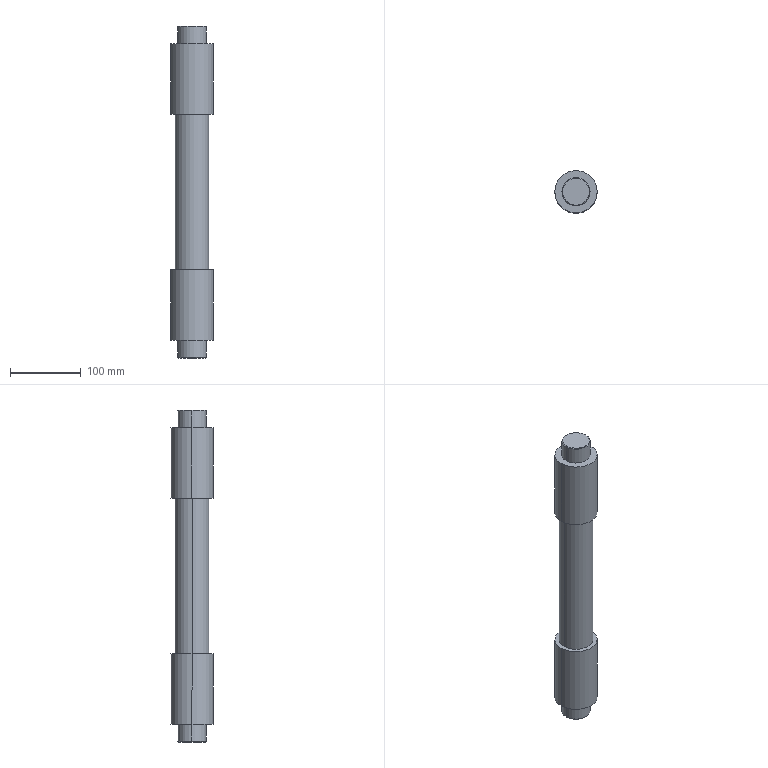Part | SolidWorks | features ICE 2, RevCut 2, Extrusion 1 | 1 solid | 20 faces | box 60 x 60 x 470 mm | volume 1026298 mm3 | cylinder 10 | plane 6 | cone 4 | commonest cylinder face diameters 40 x4 60 x4 48 x2
STEP:
#1=CARTESIAN_POINT('',(19.,0.,0.));
#2=VERTEX_POINT('',#1);
#3=CARTESIAN_POINT('',(-19.,0.,0.));
#4=VERTEX_POINT('',#3);
#5=CARTESIAN_POINT('',(0.,0.,0.));
#6=DIRECTION('',(0.,0.,1.));
#7=DIRECTION('',(1.,0.,0.));
#8=AXIS2_PLACEMENT_3D('',#5,#6,#7);
#9=CIRCLE('',#8,19.);
#10=EDGE_CURVE('',#2,#4,#9,.T.);
#11=ORIENTED_EDGE('',*,*,#10,.T.);
#12=CARTESIAN_POINT('',(-20.,0.,1.));
#13=VERTEX_POINT('',#12);
#14=CARTESIAN_POINT('',(-20.,0.,1.));
#15=DIRECTION('',(-0.7071,0.,0.7071));
#16=VECTOR('',#15,1000.);
#17=LINE('',#14,#16);
#18=EDGE_CURVE('',#4,#13,#17,.T.);
#19=ORIENTED_EDGE('',*,*,#18,.T.);
#20=CARTESIAN_POINT('',(20.,0.,1.));
#21=VERTEX_POINT('',#20);
#22=CARTESIAN_POINT('',(0.,0.,1.));
#23=DIRECTION('',(0.,0.,1.));
#24=DIRECTION('',(1.,0.,0.));
#25=AXIS2_PLACEMENT_3D('',#22,#23,#24);
#26=CIRCLE('',#25,20.);
#27=EDGE_CURVE('',#21,#13,#26,.T.);
#28=ORIENTED_EDGE('',*,*,#27,.F.);
#29=CARTESIAN_POINT('',(20.,0.,1.));
#30=DIRECTION('',(0.7071,0.,0.7071));
#31=VECTOR('',#30,1000.);
#32=LINE('',#29,#31);
#33=EDGE_CURVE('',#2,#21,#32,.T.);
#34=ORIENTED_EDGE('',*,*,#33,.F.);
#35=EDGE_LOOP('',(#11,#19,#28,#34));
#36=FACE_OUTER_BOUND('',#35,.T.);
#37=CARTESIAN_POINT('',(0.,0.,1.));
#38=DIRECTION('',(0.,0.,1.));
#39=DIRECTION('',(1.,0.,0.));
#40=AXIS2_PLACEMENT_3D('',#37,#38,#39);
#41=CONICAL_SURFACE('',#40,20.,0.7854);
#42=ADVANCED_FACE('',(#36),#41,.T.);
#43=CARTESIAN_POINT('',(19.,0.,470.));
#44=VERTEX_POINT('',#43);
#45=CARTESIAN_POINT('',(-19.,0.,470.));
#46=VERTEX_POINT('',#45);
#47=CARTESIAN_POINT('',(0.,0.,470.));
#48=DIRECTION('',(0.,0.,1.));
#49=DIRECTION('',(1.,0.,0.));
#50=AXIS2_PLACEMENT_3D('',#47,#48,#49);
#51=CIRCLE('',#50,19.);
#52=EDGE_CURVE('',#44,#46,#51,.T.);
#53=ORIENTED_EDGE('',*,*,#52,.F.);
#54=CARTESIAN_POINT('',(20.,0.,469.));
#55=VERTEX_POINT('',#54);
#56=CARTESIAN_POINT('',(20.,0.,469.));
#57=DIRECTION('',(0.7071,0.,-0.7071));
#58=VECTOR('',#57,1000.);
#59=LINE('',#56,#58);
#60=EDGE_CURVE('',#44,#55,#59,.T.);
#61=ORIENTED_EDGE('',*,*,#60,.T.);
#62=CARTESIAN_POINT('',(-20.,0.,469.));
#63=VERTEX_POINT('',#62);
#64=CARTESIAN_POINT('',(0.,0.,469.));
#65=DIRECTION('',(0.,0.,1.));
#66=DIRECTION('',(1.,0.,0.));
#67=AXIS2_PLACEMENT_3D('',#64,#65,#66);
#68=CIRCLE('',#67,20.);
#69=EDGE_CURVE('',#55,#63,#68,.T.);
#70=ORIENTED_EDGE('',*,*,#69,.T.);
#71=CARTESIAN_POINT('',(-20.,0.,469.));
#72=DIRECTION('',(-0.7071,0.,-0.7071));
#73=VECTOR('',#72,1000.);
#74=LINE('',#71,#73);
#75=EDGE_CURVE('',#46,#63,#74,.T.);
#76=ORIENTED_EDGE('',*,*,#75,.F.);
#77=EDGE_LOOP('',(#53,#61,#70,#76));
#78=FACE_OUTER_BOUND('',#77,.T.);
#79=CARTESIAN_POINT('',(0.,0.,469.));
#80=DIRECTION('',(0.,0.,-1.));
#81=DIRECTION('',(-1.,0.,0.));
#82=AXIS2_PLACEMENT_3D('',#79,#80,#81);
#83=CONICAL_SURFACE('',#82,20.,0.7854);
#84=ADVANCED_FACE('',(#78),#83,.T.);
#85=CARTESIAN_POINT('',(30.,0.,125.));
#86=VERTEX_POINT('',#85);
#87=CARTESIAN_POINT('',(-30.,0.,125.));
#88=VERTEX_POINT('',#87);
#89=CARTESIAN_POINT('',(0.,0.,125.));
#90=DIRECTION('',(0.,0.,1.));
#91=DIRECTION('',(1.,0.,0.));
#92=AXIS2_PLACEMENT_3D('',#89,#90,#91);
#93=CIRCLE('',#92,30.);
#94=EDGE_CURVE('',#86,#88,#93,.T.);
#95=ORIENTED_EDGE('',*,*,#94,.F.);
#96=CARTESIAN_POINT('',(30.,0.,25.));
#97=VERTEX_POINT('',#96);
#98=CARTESIAN_POINT('',(30.,0.,470.));
#99=DIRECTION('',(0.,0.,-1.));
#100=VECTOR('',#99,1000.);
#101=LINE('',#98,#100);
#102=EDGE_CURVE('',#86,#97,#101,.T.);
#103=ORIENTED_EDGE('',*,*,#102,.T.);
#104=CARTESIAN_POINT('',(-30.,0.,25.));
#105=VERTEX_POINT('',#104);
#106=CARTESIAN_POINT('',(0.,0.,25.));
#107=DIRECTION('',(0.,0.,-1.));
#108=DIRECTION('',(-1.,0.,0.));
#109=AXIS2_PLACEMENT_3D('',#106,#107,#108);
#110=CIRCLE('',#109,30.);
#111=EDGE_CURVE('',#105,#97,#110,.T.);
#112=ORIENTED_EDGE('',*,*,#111,.F.);
#113=CARTESIAN_POINT('',(-30.,0.,470.));
#114=DIRECTION('',(0.,0.,-1.));
#115=VECTOR('',#114,1000.);
#116=LINE('',#113,#115);
#117=EDGE_CURVE('',#88,#105,#116,.T.);
#118=ORIENTED_EDGE('',*,*,#117,.F.);
#119=EDGE_LOOP('',(#95,#103,#112,#118));
#120=FACE_OUTER_BOUND('',#119,.T.);
#121=CARTESIAN_POINT('',(0.,0.,470.));
#122=DIRECTION('',(0.,0.,-1.));
#123=DIRECTION('',(-1.,0.,0.));
#124=AXIS2_PLACEMENT_3D('',#121,#122,#123);
#125=CYLINDRICAL_SURFACE('',#124,30.);
#126=ADVANCED_FACE('',(#120),#125,.T.);
#127=CARTESIAN_POINT('',(24.,0.,125.));
#128=VERTEX_POINT('',#127);
#129=CARTESIAN_POINT('',(-24.,0.,125.));
#130=VERTEX_POINT('',#129);
#131=CARTESIAN_POINT('',(0.,0.,125.));
#132=DIRECTION('',(0.,0.,1.));
#133=DIRECTION('',(1.,0.,0.));
#134=AXIS2_PLACEMENT_3D('',#131,#132,#133);
#135=CIRCLE('',#134,24.);
#136=EDGE_CURVE('',#128,#130,#135,.T.);
#137=ORIENTED_EDGE('',*,*,#136,.T.);
#138=CARTESIAN_POINT('',(-24.,0.,345.));
#139=VERTEX_POINT('',#138);
#140=CARTESIAN_POINT('',(-24.,0.,345.));
#141=DIRECTION('',(0.,0.,1.));
#142=VECTOR('',#141,1000.);
#143=LINE('',#140,#142);
#144=EDGE_CURVE('',#130,#139,#143,.T.);
#145=ORIENTED_EDGE('',*,*,#144,.T.);
#146=CARTESIAN_POINT('',(24.,0.,345.));
#147=VERTEX_POINT('',#146);
#148=CARTESIAN_POINT('',(0.,0.,345.));
#149=DIRECTION('',(0.,0.,1.));
#150=DIRECTION('',(1.,0.,0.));
#151=AXIS2_PLACEMENT_3D('',#148,#149,#150);
#152=CIRCLE('',#151,24.);
#153=EDGE_CURVE('',#147,#139,#152,.T.);
#154=ORIENTED_EDGE('',*,*,#153,.F.);
#155=CARTESIAN_POINT('',(24.,0.,345.));
#156=DIRECTION('',(0.,0.,1.));
#157=VECTOR('',#156,1000.);
#158=LINE('',#155,#157);
#159=EDGE_CURVE('',#128,#147,#158,.T.);
#160=ORIENTED_EDGE('',*,*,#159,.F.);
#161=EDGE_LOOP('',(#137,#145,#154,#160));
#162=FACE_OUTER_BOUND('',#161,.T.);
#163=CARTESIAN_POINT('',(0.,0.,345.));
#164=DIRECTION('',(0.,0.,1.));
#165=DIRECTION('',(1.,0.,0.));
#166=AXIS2_PLACEMENT_3D('',#163,#164,#165);
#167=CYLINDRICAL_SURFACE('',#166,24.);
#168=ADVANCED_FACE('',(#162),#167,.T.);
#169=CARTESIAN_POINT('',(20.,0.,445.));
#170=VERTEX_POINT('',#169);
#171=CARTESIAN_POINT('',(-20.,0.,445.));
#172=VERTEX_POINT('',#171);
#173=CARTESIAN_POINT('',(0.,0.,445.));
#174=DIRECTION('',(0.,0.,1.));
#175=DIRECTION('',(1.,0.,0.));
#176=AXIS2_PLACEMENT_3D('',#173,#174,#175);
#177=CIRCLE('',#176,20.);
#178=EDGE_CURVE('',#170,#172,#177,.T.);
#179=ORIENTED_EDGE('',*,*,#178,.T.);
#180=CARTESIAN_POINT('',(-20.,0.,445.));
#181=DIRECTION('',(0.,0.,1.));
#182=VECTOR('',#181,1000.);
#183=LINE('',#180,#182);
#184=EDGE_CURVE('',#172,#63,#183,.T.);
#185=ORIENTED_EDGE('',*,*,#184,.T.);
#186=ORIENTED_EDGE('',*,*,#69,.F.);
#187=CARTESIAN_POINT('',(20.,0.,445.));
#188=DIRECTION('',(0.,0.,1.));
#189=VECTOR('',#188,1000.);
#190=LINE('',#187,#189);
#191=EDGE_CURVE('',#170,#55,#190,.T.);
#192=ORIENTED_EDGE('',*,*,#191,.F.);
#193=EDGE_LOOP('',(#179,#185,#186,#192));
#194=FACE_OUTER_BOUND('',#193,.T.);
#195=CARTESIAN_POINT('',(0.,0.,445.));
#196=DIRECTION('',(0.,0.,1.));
#197=DIRECTION('',(1.,0.,0.));
#198=AXIS2_PLACEMENT_3D('',#195,#196,#197);
#199=CYLINDRICAL_SURFACE('',#198,20.);
#200=ADVANCED_FACE('',(#194),#199,.T.);
#201=CARTESIAN_POINT('',(30.,0.,445.));
#202=VERTEX_POINT('',#201);
#203=CARTESIAN_POINT('',(-30.,0.,445.));
#204=VERTEX_POINT('',#203);
#205=CARTESIAN_POINT('',(0.,0.,445.));
#206=DIRECTION('',(0.,0.,1.));
#207=DIRECTION('',(1.,0.,0.));
#208=AXIS2_PLACEMENT_3D('',#205,#206,#207);
#209=CIRCLE('',#208,30.);
#210=EDGE_CURVE('',#202,#204,#209,.T.);
#211=ORIENTED_EDGE('',*,*,#210,.F.);
#212=CARTESIAN_POINT('',(30.,0.,345.));
#213=VERTEX_POINT('',#212);
#214=CARTESIAN_POINT('',(30.,0.,470.));
#215=DIRECTION('',(0.,0.,-1.));
#216=VECTOR('',#215,1000.);
#217=LINE('',#214,#216);
#218=EDGE_CURVE('',#202,#213,#217,.T.);
#219=ORIENTED_EDGE('',*,*,#218,.T.);
#220=CARTESIAN_POINT('',(-30.,0.,345.));
#221=VERTEX_POINT('',#220);
#222=CARTESIAN_POINT('',(0.,0.,345.));
#223=DIRECTION('',(0.,0.,1.));
#224=DIRECTION('',(1.,0.,0.));
#225=AXIS2_PLACEMENT_3D('',#222,#223,#224);
#226=CIRCLE('',#225,30.);
#227=EDGE_CURVE('',#213,#221,#226,.T.);
#228=ORIENTED_EDGE('',*,*,#227,.T.);
#229=CARTESIAN_POINT('',(-30.,0.,470.));
#230=DIRECTION('',(0.,0.,-1.));
#231=VECTOR('',#230,1000.);
#232=LINE('',#229,#231);
#233=EDGE_CURVE('',#204,#221,#232,.T.);
#234=ORIENTED_EDGE('',*,*,#233,.F.);
#235=EDGE_LOOP('',(#211,#219,#228,#234));
#236=FACE_OUTER_BOUND('',#235,.T.);
#237=CARTESIAN_POINT('',(0.,0.,470.));
#238=DIRECTION('',(0.,0.,-1.));
#239=DIRECTION('',(-1.,0.,0.));
#240=AXIS2_PLACEMENT_3D('',#237,#238,#239);
#241=CYLINDRICAL_SURFACE('',#240,30.);
#242=ADVANCED_FACE('',(#236),#241,.T.);
#243=CARTESIAN_POINT('',(-20.,0.,25.));
#244=VERTEX_POINT('',#243);
#245=CARTESIAN_POINT('',(20.,0.,25.));
#246=VERTEX_POINT('',#245);
#247=CARTESIAN_POINT('',(0.,0.,25.));
#248=DIRECTION('',(0.,0.,-1.));
#249=DIRECTION('',(-1.,0.,0.));
#250=AXIS2_PLACEMENT_3D('',#247,#248,#249);
#251=CIRCLE('',#250,20.);
#252=EDGE_CURVE('',#244,#246,#251,.T.);
#253=ORIENTED_EDGE('',*,*,#252,.T.);
#254=CARTESIAN_POINT('',(20.,0.,25.));
#255=DIRECTION('',(0.,0.,-1.));
#256=VECTOR('',#255,1000.);
#257=LINE('',#254,#256);
#258=EDGE_CURVE('',#246,#21,#257,.T.);
#259=ORIENTED_EDGE('',*,*,#258,.T.);
#260=ORIENTED_EDGE('',*,*,#27,.T.);
#261=CARTESIAN_POINT('',(-20.,0.,25.));
#262=DIRECTION('',(0.,0.,-1.));
#263=VECTOR('',#262,1000.);
#264=LINE('',#261,#263);
#265=EDGE_CURVE('',#244,#13,#264,.T.);
#266=ORIENTED_EDGE('',*,*,#265,.F.);
#267=EDGE_LOOP('',(#253,#259,#260,#266));
#268=FACE_OUTER_BOUND('',#267,.T.);
#269=CARTESIAN_POINT('',(0.,0.,25.));
#270=DIRECTION('',(0.,0.,-1.));
#271=DIRECTION('',(-1.,0.,0.));
#272=AXIS2_PLACEMENT_3D('',#269,#270,#271);
#273=CYLINDRICAL_SURFACE('',#272,20.);
#274=ADVANCED_FACE('',(#268),#273,.T.);
#275=ORIENTED_EDGE('',*,*,#258,.F.);
#276=CARTESIAN_POINT('',(0.,0.,25.));
#277=DIRECTION('',(0.,0.,-1.));
#278=DIRECTION('',(-1.,0.,0.));
#279=AXIS2_PLACEMENT_3D('',#276,#277,#278);
#280=CIRCLE('',#279,20.);
#281=EDGE_CURVE('',#246,#244,#280,.T.);
#282=ORIENTED_EDGE('',*,*,#281,.T.);
#283=ORIENTED_EDGE('',*,*,#265,.T.);
#284=CARTESIAN_POINT('',(0.,0.,1.));
#285=DIRECTION('',(0.,0.,1.));
#286=DIRECTION('',(1.,0.,0.));
#287=AXIS2_PLACEMENT_3D('',#284,#285,#286);
#288=CIRCLE('',#287,20.);
#289=EDGE_CURVE('',#13,#21,#288,.T.);
#290=ORIENTED_EDGE('',*,*,#289,.T.);
#291=EDGE_LOOP('',(#275,#282,#283,#290));
#292=FACE_OUTER_BOUND('',#291,.T.);
#293=CARTESIAN_POINT('',(0.,0.,25.));
#294=DIRECTION('',(0.,0.,-1.));
#295=DIRECTION('',(-1.,0.,0.));
#296=AXIS2_PLACEMENT_3D('',#293,#294,#295);
#297=CYLINDRICAL_SURFACE('',#296,20.);
#298=ADVANCED_FACE('',(#292),#297,.T.);
#299=ORIENTED_EDGE('',*,*,#218,.F.);
#300=CARTESIAN_POINT('',(0.,0.,445.));
#301=DIRECTION('',(0.,0.,1.));
#302=DIRECTION('',(1.,0.,0.));
#303=AXIS2_PLACEMENT_3D('',#300,#301,#302);
#304=CIRCLE('',#303,30.);
#305=EDGE_CURVE('',#204,#202,#304,.T.);
#306=ORIENTED_EDGE('',*,*,#305,.F.);
#307=ORIENTED_EDGE('',*,*,#233,.T.);
#308=CARTESIAN_POINT('',(0.,0.,345.));
#309=DIRECTION('',(0.,0.,1.));
#310=DIRECTION('',(1.,0.,0.));
#311=AXIS2_PLACEMENT_3D('',#308,#309,#310);
#312=CIRCLE('',#311,30.);
#313=EDGE_CURVE('',#221,#213,#312,.T.);
#314=ORIENTED_EDGE('',*,*,#313,.T.);
#315=EDGE_LOOP('',(#299,#306,#307,#314));
#316=FACE_OUTER_BOUND('',#315,.T.);
#317=CARTESIAN_POINT('',(0.,0.,470.));
#318=DIRECTION('',(0.,0.,-1.));
#319=DIRECTION('',(-1.,0.,0.));
#320=AXIS2_PLACEMENT_3D('',#317,#318,#319);
#321=CYLINDRICAL_SURFACE('',#320,30.);
#322=ADVANCED_FACE('',(#316),#321,.T.);
#323=ORIENTED_EDGE('',*,*,#178,.F.);
#324=CARTESIAN_POINT('',(0.,0.,445.));
#325=DIRECTION('',(0.,0.,1.));
#326=DIRECTION('',(1.,0.,0.));
#327=AXIS2_PLACEMENT_3D('',#324,#325,#326);
#328=CIRCLE('',#327,20.);
#329=EDGE_CURVE('',#172,#170,#328,.T.);
#330=ORIENTED_EDGE('',*,*,#329,.F.);
#331=EDGE_LOOP('',(#323,#330));
#332=FACE_BOUND('',#331,.T.);
#333=ORIENTED_EDGE('',*,*,#305,.T.);
#334=ORIENTED_EDGE('',*,*,#210,.T.);
#335=EDGE_LOOP('',(#333,#334));
#336=FACE_OUTER_BOUND('',#335,.T.);
#337=CARTESIAN_POINT('',(0.,0.,445.));
#338=DIRECTION('',(0.,0.,1.));
#339=DIRECTION('',(1.,0.,0.));
#340=AXIS2_PLACEMENT_3D('',#337,#338,#339);
#341=PLANE('',#340);
#342=ADVANCED_FACE('',(#332,#336),#341,.T.);
#343=ORIENTED_EDGE('',*,*,#184,.F.);
#344=ORIENTED_EDGE('',*,*,#329,.T.);
#345=ORIENTED_EDGE('',*,*,#191,.T.);
#346=CARTESIAN_POINT('',(0.,0.,469.));
#347=DIRECTION('',(0.,0.,1.));
#348=DIRECTION('',(1.,0.,0.));
#349=AXIS2_PLACEMENT_3D('',#346,#347,#348);
#350=CIRCLE('',#349,20.);
#351=EDGE_CURVE('',#63,#55,#350,.T.);
#352=ORIENTED_EDGE('',*,*,#351,.F.);
#353=EDGE_LOOP('',(#343,#344,#345,#352));
#354=FACE_OUTER_BOUND('',#353,.T.);
#355=CARTESIAN_POINT('',(0.,0.,445.));
#356=DIRECTION('',(0.,0.,1.));
#357=DIRECTION('',(1.,0.,0.));
#358=AXIS2_PLACEMENT_3D('',#355,#356,#357);
#359=CYLINDRICAL_SURFACE('',#358,20.);
#360=ADVANCED_FACE('',(#354),#359,.T.);
#361=ORIENTED_EDGE('',*,*,#153,.T.);
#362=CARTESIAN_POINT('',(0.,0.,345.));
#363=DIRECTION('',(0.,0.,1.));
#364=DIRECTION('',(1.,0.,0.));
#365=AXIS2_PLACEMENT_3D('',#362,#363,#364);
#366=CIRCLE('',#365,24.);
#367=EDGE_CURVE('',#139,#147,#366,.T.);
#368=ORIENTED_EDGE('',*,*,#367,.T.);
#369=EDGE_LOOP('',(#361,#368));
#370=FACE_BOUND('',#369,.T.);
#371=ORIENTED_EDGE('',*,*,#313,.F.);
#372=ORIENTED_EDGE('',*,*,#227,.F.);
#373=EDGE_LOOP('',(#371,#372));
#374=FACE_OUTER_BOUND('',#373,.T.);
#375=CARTESIAN_POINT('',(0.,0.,345.));
#376=DIRECTION('',(0.,0.,-1.));
#377=DIRECTION('',(-1.,0.,0.));
#378=AXIS2_PLACEMENT_3D('',#375,#376,#377);
#379=PLANE('',#378);
#380=ADVANCED_FACE('',(#370,#374),#379,.T.);
#381=ORIENTED_EDGE('',*,*,#144,.F.);
#382=CARTESIAN_POINT('',(0.,0.,125.));
#383=DIRECTION('',(0.,0.,1.));
#384=DIRECTION('',(1.,0.,0.));
#385=AXIS2_PLACEMENT_3D('',#382,#383,#384);
#386=CIRCLE('',#385,24.);
#387=EDGE_CURVE('',#130,#128,#386,.T.);
#388=ORIENTED_EDGE('',*,*,#387,.T.);
#389=ORIENTED_EDGE('',*,*,#159,.T.);
#390=ORIENTED_EDGE('',*,*,#367,.F.);
#391=EDGE_LOOP('',(#381,#388,#389,#390));
#392=FACE_OUTER_BOUND('',#391,.T.);
#393=CARTESIAN_POINT('',(0.,0.,345.));
#394=DIRECTION('',(0.,0.,1.));
#395=DIRECTION('',(1.,0.,0.));
#396=AXIS2_PLACEMENT_3D('',#393,#394,#395);
#397=CYLINDRICAL_SURFACE('',#396,24.);
#398=ADVANCED_FACE('',(#392),#397,.T.);
#399=ORIENTED_EDGE('',*,*,#136,.F.);
#400=ORIENTED_EDGE('',*,*,#387,.F.);
#401=EDGE_LOOP('',(#399,#400));
#402=FACE_BOUND('',#401,.T.);
#403=CARTESIAN_POINT('',(0.,0.,125.));
#404=DIRECTION('',(0.,0.,1.));
#405=DIRECTION('',(1.,0.,0.));
#406=AXIS2_PLACEMENT_3D('',#403,#404,#405);
#407=CIRCLE('',#406,30.);
#408=EDGE_CURVE('',#88,#86,#407,.T.);
#409=ORIENTED_EDGE('',*,*,#408,.T.);
#410=ORIENTED_EDGE('',*,*,#94,.T.);
#411=EDGE_LOOP('',(#409,#410));
#412=FACE_OUTER_BOUND('',#411,.T.);
#413=CARTESIAN_POINT('',(0.,0.,125.));
#414=DIRECTION('',(0.,0.,-1.));
#415=DIRECTION('',(-1.,0.,0.));
#416=AXIS2_PLACEMENT_3D('',#413,#414,#415);
#417=PLANE('',#416);
#418=ADVANCED_FACE('',(#402,#412),#417,.F.);
#419=ORIENTED_EDGE('',*,*,#252,.F.);
#420=ORIENTED_EDGE('',*,*,#281,.F.);
#421=EDGE_LOOP('',(#419,#420));
#422=FACE_BOUND('',#421,.T.);
#423=ORIENTED_EDGE('',*,*,#111,.T.);
#424=CARTESIAN_POINT('',(0.,0.,25.));
#425=DIRECTION('',(0.,0.,-1.));
#426=DIRECTION('',(-1.,0.,0.));
#427=AXIS2_PLACEMENT_3D('',#424,#425,#426);
#428=CIRCLE('',#427,30.);
#429=EDGE_CURVE('',#97,#105,#428,.T.);
#430=ORIENTED_EDGE('',*,*,#429,.T.);
#431=EDGE_LOOP('',(#423,#430));
#432=FACE_OUTER_BOUND('',#431,.T.);
#433=CARTESIAN_POINT('',(0.,0.,25.));
#434=DIRECTION('',(0.,0.,-1.));
#435=DIRECTION('',(-1.,0.,0.));
#436=AXIS2_PLACEMENT_3D('',#433,#434,#435);
#437=PLANE('',#436);
#438=ADVANCED_FACE('',(#422,#432),#437,.T.);
#439=ORIENTED_EDGE('',*,*,#102,.F.);
#440=ORIENTED_EDGE('',*,*,#408,.F.);
#441=ORIENTED_EDGE('',*,*,#117,.T.);
#442=ORIENTED_EDGE('',*,*,#429,.F.);
#443=EDGE_LOOP('',(#439,#440,#441,#442));
#444=FACE_OUTER_BOUND('',#443,.T.);
#445=CARTESIAN_POINT('',(0.,0.,470.));
#446=DIRECTION('',(0.,0.,-1.));
#447=DIRECTION('',(-1.,0.,0.));
#448=AXIS2_PLACEMENT_3D('',#445,#446,#447);
#449=CYLINDRICAL_SURFACE('',#448,30.);
#450=ADVANCED_FACE('',(#444),#449,.T.);
#451=ORIENTED_EDGE('',*,*,#60,.F.);
#452=CARTESIAN_POINT('',(0.,0.,470.));
#453=DIRECTION('',(0.,0.,1.));
#454=DIRECTION('',(1.,0.,0.));
#455=AXIS2_PLACEMENT_3D('',#452,#453,#454);
#456=CIRCLE('',#455,19.);
#457=EDGE_CURVE('',#46,#44,#456,.T.);
#458=ORIENTED_EDGE('',*,*,#457,.F.);
#459=ORIENTED_EDGE('',*,*,#75,.T.);
#460=ORIENTED_EDGE('',*,*,#351,.T.);
#461=EDGE_LOOP('',(#451,#458,#459,#460));
#462=FACE_OUTER_BOUND('',#461,.T.);
#463=CARTESIAN_POINT('',(0.,0.,469.));
#464=DIRECTION('',(0.,0.,-1.));
#465=DIRECTION('',(-1.,0.,0.));
#466=AXIS2_PLACEMENT_3D('',#463,#464,#465);
#467=CONICAL_SURFACE('',#466,20.,0.7854);
#468=ADVANCED_FACE('',(#462),#467,.T.);
#469=ORIENTED_EDGE('',*,*,#457,.T.);
#470=ORIENTED_EDGE('',*,*,#52,.T.);
#471=EDGE_LOOP('',(#469,#470));
#472=FACE_OUTER_BOUND('',#471,.T.);
#473=CARTESIAN_POINT('',(0.,0.,470.));
#474=DIRECTION('',(0.,0.,1.));
#475=DIRECTION('',(1.,0.,0.));
#476=AXIS2_PLACEMENT_3D('',#473,#474,#475);
#477=PLANE('',#476);
#478=ADVANCED_FACE('',(#472),#477,.T.);
#479=ORIENTED_EDGE('',*,*,#18,.F.);
#480=CARTESIAN_POINT('',(0.,0.,0.));
#481=DIRECTION('',(0.,0.,1.));
#482=DIRECTION('',(1.,0.,0.));
#483=AXIS2_PLACEMENT_3D('',#480,#481,#482);
#484=CIRCLE('',#483,19.);
#485=EDGE_CURVE('',#4,#2,#484,.T.);
#486=ORIENTED_EDGE('',*,*,#485,.T.);
#487=ORIENTED_EDGE('',*,*,#33,.T.);
#488=ORIENTED_EDGE('',*,*,#289,.F.);
#489=EDGE_LOOP('',(#479,#486,#487,#488));
#490=FACE_OUTER_BOUND('',#489,.T.);
#491=CARTESIAN_POINT('',(0.,0.,1.));
#492=DIRECTION('',(0.,0.,1.));
#493=DIRECTION('',(1.,0.,0.));
#494=AXIS2_PLACEMENT_3D('',#491,#492,#493);
#495=CONICAL_SURFACE('',#494,20.,0.7854);
#496=ADVANCED_FACE('',(#490),#495,.T.);
#497=ORIENTED_EDGE('',*,*,#10,.F.);
#498=ORIENTED_EDGE('',*,*,#485,.F.);
#499=EDGE_LOOP('',(#497,#498));
#500=FACE_OUTER_BOUND('',#499,.T.);
#501=CARTESIAN_POINT('',(0.,0.,0.));
#502=DIRECTION('',(0.,0.,1.));
#503=DIRECTION('',(1.,0.,0.));
#504=AXIS2_PLACEMENT_3D('',#501,#502,#503);
#505=PLANE('',#504);
#506=ADVANCED_FACE('',(#500),#505,.F.);
#507=CLOSED_SHELL('',(#42,#84,#126,#168,#200,#242,#274,#298,#322,#342,#360,#380,#398,#418,#438,#450,#468,#478,#496,#506));
#508=MANIFOLD_SOLID_BREP('',#507);
#509=CARTESIAN_POINT('',(0.,0.,0.));
#510=DIRECTION('',(0.,0.,1.));
#511=DIRECTION('',(1.,0.,0.));
#512=AXIS2_PLACEMENT_3D('',#509,#510,#511);
#513=(LENGTH_UNIT()NAMED_UNIT(*)SI_UNIT(.MILLI.,.METRE.));
#514=UNCERTAINTY_MEASURE_WITH_UNIT(LENGTH_MEASURE(0.00001),#513,'','');
#515=(NAMED_UNIT(*)PLANE_ANGLE_UNIT()SI_UNIT($,.RADIAN.));
#516=(NAMED_UNIT(*)SI_UNIT($,.STERADIAN.)SOLID_ANGLE_UNIT());
#517=(GEOMETRIC_REPRESENTATION_CONTEXT(3)GLOBAL_UNCERTAINTY_ASSIGNED_CONTEXT((#514))GLOBAL_UNIT_ASSIGNED_CONTEXT((#513,#515,#516))REPRESENTATION_CONTEXT('',''));
#518=ADVANCED_BREP_SHAPE_REPRESENTATION('',(#508,#512),#517);